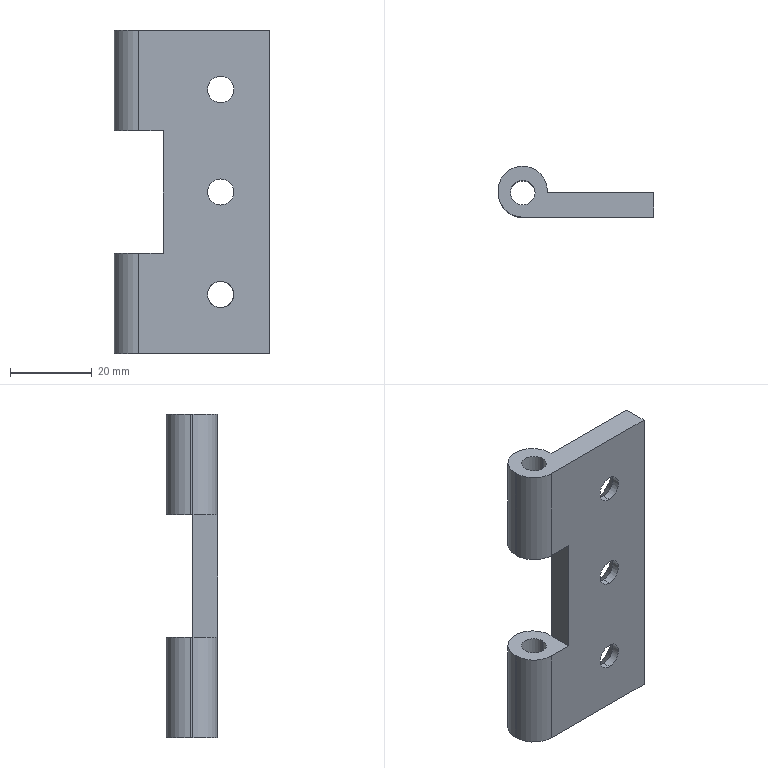Part | SolidWorks | features BaseBody 1 | 1 solid | 32 faces | box 38 x 12.5 x 79 mm | volume 15890 mm3 | cylinder 14 | plane 12 | cone 6 | commonest cylinder face diameters 6.4 x6 6 x4 12 x4
STEP:
#1=CARTESIAN_POINT('',(-20.,1556.,1039.));
#2=VERTEX_POINT('',#1);
#3=CARTESIAN_POINT('',(-26.,1556.,1039.));
#4=VERTEX_POINT('',#3);
#5=CARTESIAN_POINT('',(-23.,1556.,1039.));
#6=DIRECTION('',(0.,0.,-1.));
#7=DIRECTION('',(1.,0.,0.));
#8=AXIS2_PLACEMENT_3D('',#5,#6,#7);
#9=CIRCLE('',#8,3.);
#10=EDGE_CURVE('',#2,#4,#9,.T.);
#11=ORIENTED_EDGE('',*,*,#10,.T.);
#12=CARTESIAN_POINT('',(-26.,1556.,1063.5));
#13=VERTEX_POINT('',#12);
#14=CARTESIAN_POINT('',(-26.,1556.,1039.));
#15=DIRECTION('',(0.,0.,1.));
#16=VECTOR('',#15,1000.);
#17=LINE('',#14,#16);
#18=EDGE_CURVE('',#4,#13,#17,.T.);
#19=ORIENTED_EDGE('',*,*,#18,.T.);
#20=CARTESIAN_POINT('',(-20.,1556.,1063.5));
#21=VERTEX_POINT('',#20);
#22=CARTESIAN_POINT('',(-23.,1556.,1063.5));
#23=DIRECTION('',(0.,0.,1.));
#24=DIRECTION('',(1.,0.,0.));
#25=AXIS2_PLACEMENT_3D('',#22,#23,#24);
#26=CIRCLE('',#25,3.);
#27=EDGE_CURVE('',#13,#21,#26,.T.);
#28=ORIENTED_EDGE('',*,*,#27,.T.);
#29=CARTESIAN_POINT('',(-20.,1556.,1039.));
#30=DIRECTION('',(0.,0.,1.));
#31=VECTOR('',#30,1000.);
#32=LINE('',#29,#31);
#33=EDGE_CURVE('',#2,#21,#32,.T.);
#34=ORIENTED_EDGE('',*,*,#33,.F.);
#35=EDGE_LOOP('',(#11,#19,#28,#34));
#36=FACE_OUTER_BOUND('',#35,.T.);
#37=CARTESIAN_POINT('',(-23.,1556.,1039.));
#38=DIRECTION('',(0.,0.,1.));
#39=DIRECTION('',(1.,0.,0.));
#40=AXIS2_PLACEMENT_3D('',#37,#38,#39);
#41=CYLINDRICAL_SURFACE('',#40,3.);
#42=ADVANCED_FACE('',(#36),#41,.F.);
#43=CARTESIAN_POINT('',(-3.,1552.,1081.7));
#44=VERTEX_POINT('',#43);
#45=CARTESIAN_POINT('',(-3.,1552.,1075.3));
#46=VERTEX_POINT('',#45);
#47=CARTESIAN_POINT('',(-3.,1552.,1078.5));
#48=DIRECTION('',(0.,-1.,0.));
#49=DIRECTION('',(0.,0.,-1.));
#50=AXIS2_PLACEMENT_3D('',#47,#48,#49);
#51=CIRCLE('',#50,3.2);
#52=EDGE_CURVE('',#44,#46,#51,.T.);
#53=ORIENTED_EDGE('',*,*,#52,.T.);
#54=CARTESIAN_POINT('',(-3.,1556.,1071.3));
#55=VERTEX_POINT('',#54);
#56=CARTESIAN_POINT('',(-3.,1552.,1075.3));
#57=DIRECTION('',(0.,0.7071,-0.7071));
#58=VECTOR('',#57,1000.);
#59=LINE('',#56,#58);
#60=EDGE_CURVE('',#46,#55,#59,.T.);
#61=ORIENTED_EDGE('',*,*,#60,.T.);
#62=CARTESIAN_POINT('',(-3.,1556.,1085.7));
#63=VERTEX_POINT('',#62);
#64=CARTESIAN_POINT('',(-3.,1556.,1078.5));
#65=DIRECTION('',(0.,-1.,0.));
#66=DIRECTION('',(0.,0.,1.));
#67=AXIS2_PLACEMENT_3D('',#64,#65,#66);
#68=CIRCLE('',#67,7.2);
#69=EDGE_CURVE('',#63,#55,#68,.T.);
#70=ORIENTED_EDGE('',*,*,#69,.F.);
#71=CARTESIAN_POINT('',(-3.,1552.,1081.7));
#72=DIRECTION('',(0.,0.7071,0.7071));
#73=VECTOR('',#72,1000.);
#74=LINE('',#71,#73);
#75=EDGE_CURVE('',#44,#63,#74,.T.);
#76=ORIENTED_EDGE('',*,*,#75,.F.);
#77=EDGE_LOOP('',(#53,#61,#70,#76));
#78=FACE_OUTER_BOUND('',#77,.T.);
#79=CARTESIAN_POINT('',(-3.,1552.,1078.5));
#80=DIRECTION('',(0.,1.,0.));
#81=DIRECTION('',(0.,0.,1.));
#82=AXIS2_PLACEMENT_3D('',#79,#80,#81);
#83=CONICAL_SURFACE('',#82,3.2,0.7854);
#84=ADVANCED_FACE('',(#78),#83,.F.);
#85=CARTESIAN_POINT('',(-3.,1552.,1106.7));
#86=VERTEX_POINT('',#85);
#87=CARTESIAN_POINT('',(-3.,1552.,1100.3));
#88=VERTEX_POINT('',#87);
#89=CARTESIAN_POINT('',(-3.,1552.,1103.5));
#90=DIRECTION('',(0.,-1.,0.));
#91=DIRECTION('',(0.,0.,-1.));
#92=AXIS2_PLACEMENT_3D('',#89,#90,#91);
#93=CIRCLE('',#92,3.2);
#94=EDGE_CURVE('',#86,#88,#93,.T.);
#95=ORIENTED_EDGE('',*,*,#94,.T.);
#96=CARTESIAN_POINT('',(-3.,1556.,1096.3));
#97=VERTEX_POINT('',#96);
#98=CARTESIAN_POINT('',(-3.,1552.,1100.3));
#99=DIRECTION('',(0.,0.7071,-0.7071));
#100=VECTOR('',#99,1000.);
#101=LINE('',#98,#100);
#102=EDGE_CURVE('',#88,#97,#101,.T.);
#103=ORIENTED_EDGE('',*,*,#102,.T.);
#104=CARTESIAN_POINT('',(-3.,1556.,1110.7));
#105=VERTEX_POINT('',#104);
#106=CARTESIAN_POINT('',(-3.,1556.,1103.5));
#107=DIRECTION('',(0.,-1.,0.));
#108=DIRECTION('',(0.,0.,1.));
#109=AXIS2_PLACEMENT_3D('',#106,#107,#108);
#110=CIRCLE('',#109,7.2);
#111=EDGE_CURVE('',#105,#97,#110,.T.);
#112=ORIENTED_EDGE('',*,*,#111,.F.);
#113=CARTESIAN_POINT('',(-3.,1552.,1106.7));
#114=DIRECTION('',(0.,0.7071,0.7071));
#115=VECTOR('',#114,1000.);
#116=LINE('',#113,#115);
#117=EDGE_CURVE('',#86,#105,#116,.T.);
#118=ORIENTED_EDGE('',*,*,#117,.F.);
#119=EDGE_LOOP('',(#95,#103,#112,#118));
#120=FACE_OUTER_BOUND('',#119,.T.);
#121=CARTESIAN_POINT('',(-3.,1552.,1103.5));
#122=DIRECTION('',(0.,1.,0.));
#123=DIRECTION('',(0.,0.,1.));
#124=AXIS2_PLACEMENT_3D('',#121,#122,#123);
#125=CONICAL_SURFACE('',#124,3.2,0.7854);
#126=ADVANCED_FACE('',(#120),#125,.F.);
#127=CARTESIAN_POINT('',(-3.,1552.,1050.3));
#128=VERTEX_POINT('',#127);
#129=CARTESIAN_POINT('',(0.2,1552.,1053.5));
#130=VERTEX_POINT('',#129);
#131=CARTESIAN_POINT('',(-3.,1552.,1053.5));
#132=DIRECTION('',(0.,-1.,0.));
#133=DIRECTION('',(0.,0.,-1.));
#134=AXIS2_PLACEMENT_3D('',#131,#132,#133);
#135=CIRCLE('',#134,3.2);
#136=EDGE_CURVE('',#128,#130,#135,.T.);
#137=ORIENTED_EDGE('',*,*,#136,.T.);
#138=CARTESIAN_POINT('',(4.2,1556.,1053.5));
#139=VERTEX_POINT('',#138);
#140=CARTESIAN_POINT('',(0.2,1552.,1053.5));
#141=DIRECTION('',(0.7071,0.7071,0.));
#142=VECTOR('',#141,1000.);
#143=LINE('',#140,#142);
#144=EDGE_CURVE('',#130,#139,#143,.T.);
#145=ORIENTED_EDGE('',*,*,#144,.T.);
#146=CARTESIAN_POINT('',(-10.2,1556.,1053.5));
#147=VERTEX_POINT('',#146);
#148=CARTESIAN_POINT('',(-3.,1556.,1053.5));
#149=DIRECTION('',(0.,-1.,0.));
#150=DIRECTION('',(-1.,0.,0.));
#151=AXIS2_PLACEMENT_3D('',#148,#149,#150);
#152=CIRCLE('',#151,7.2);
#153=EDGE_CURVE('',#147,#139,#152,.T.);
#154=ORIENTED_EDGE('',*,*,#153,.F.);
#155=CARTESIAN_POINT('',(-6.2,1552.,1053.5));
#156=VERTEX_POINT('',#155);
#157=CARTESIAN_POINT('',(-6.2,1552.,1053.5));
#158=DIRECTION('',(-0.7071,0.7071,0.));
#159=VECTOR('',#158,1000.);
#160=LINE('',#157,#159);
#161=EDGE_CURVE('',#156,#147,#160,.T.);
#162=ORIENTED_EDGE('',*,*,#161,.F.);
#163=CARTESIAN_POINT('',(-3.,1552.,1053.5));
#164=DIRECTION('',(0.,-1.,0.));
#165=DIRECTION('',(0.,0.,-1.));
#166=AXIS2_PLACEMENT_3D('',#163,#164,#165);
#167=CIRCLE('',#166,3.2);
#168=EDGE_CURVE('',#156,#128,#167,.T.);
#169=ORIENTED_EDGE('',*,*,#168,.T.);
#170=EDGE_LOOP('',(#137,#145,#154,#162,#169));
#171=FACE_OUTER_BOUND('',#170,.T.);
#172=CARTESIAN_POINT('',(-3.,1552.,1053.5));
#173=DIRECTION('',(0.,1.,0.));
#174=DIRECTION('',(-1.,0.,0.));
#175=AXIS2_PLACEMENT_3D('',#172,#173,#174);
#176=CONICAL_SURFACE('',#175,3.2,0.7854);
#177=ADVANCED_FACE('',(#171),#176,.F.);
#178=CARTESIAN_POINT('',(-3.,1550.,1100.3));
#179=VERTEX_POINT('',#178);
#180=CARTESIAN_POINT('',(-3.,1550.,1106.7));
#181=VERTEX_POINT('',#180);
#182=CARTESIAN_POINT('',(-3.,1550.,1103.5));
#183=DIRECTION('',(0.,1.,0.));
#184=DIRECTION('',(0.,0.,1.));
#185=AXIS2_PLACEMENT_3D('',#182,#183,#184);
#186=CIRCLE('',#185,3.2);
#187=EDGE_CURVE('',#179,#181,#186,.T.);
#188=ORIENTED_EDGE('',*,*,#187,.F.);
#189=CARTESIAN_POINT('',(-3.,1550.,1100.3));
#190=DIRECTION('',(0.,1.,0.));
#191=VECTOR('',#190,1000.);
#192=LINE('',#189,#191);
#193=EDGE_CURVE('',#179,#88,#192,.T.);
#194=ORIENTED_EDGE('',*,*,#193,.T.);
#195=ORIENTED_EDGE('',*,*,#94,.F.);
#196=CARTESIAN_POINT('',(-3.,1550.,1106.7));
#197=DIRECTION('',(0.,1.,0.));
#198=VECTOR('',#197,1000.);
#199=LINE('',#196,#198);
#200=EDGE_CURVE('',#181,#86,#199,.T.);
#201=ORIENTED_EDGE('',*,*,#200,.F.);
#202=EDGE_LOOP('',(#188,#194,#195,#201));
#203=FACE_OUTER_BOUND('',#202,.T.);
#204=CARTESIAN_POINT('',(-3.,1550.,1103.5));
#205=DIRECTION('',(0.,1.,0.));
#206=DIRECTION('',(0.,0.,1.));
#207=AXIS2_PLACEMENT_3D('',#204,#205,#206);
#208=CYLINDRICAL_SURFACE('',#207,3.2);
#209=ADVANCED_FACE('',(#203),#208,.F.);
#210=CARTESIAN_POINT('',(-3.,1550.,1075.3));
#211=VERTEX_POINT('',#210);
#212=CARTESIAN_POINT('',(-3.,1550.,1081.7));
#213=VERTEX_POINT('',#212);
#214=CARTESIAN_POINT('',(-3.,1550.,1078.5));
#215=DIRECTION('',(0.,1.,0.));
#216=DIRECTION('',(0.,0.,1.));
#217=AXIS2_PLACEMENT_3D('',#214,#215,#216);
#218=CIRCLE('',#217,3.2);
#219=EDGE_CURVE('',#211,#213,#218,.T.);
#220=ORIENTED_EDGE('',*,*,#219,.F.);
#221=CARTESIAN_POINT('',(-3.,1550.,1075.3));
#222=DIRECTION('',(0.,1.,0.));
#223=VECTOR('',#222,1000.);
#224=LINE('',#221,#223);
#225=EDGE_CURVE('',#211,#46,#224,.T.);
#226=ORIENTED_EDGE('',*,*,#225,.T.);
#227=ORIENTED_EDGE('',*,*,#52,.F.);
#228=CARTESIAN_POINT('',(-3.,1550.,1081.7));
#229=DIRECTION('',(0.,1.,0.));
#230=VECTOR('',#229,1000.);
#231=LINE('',#228,#230);
#232=EDGE_CURVE('',#213,#44,#231,.T.);
#233=ORIENTED_EDGE('',*,*,#232,.F.);
#234=EDGE_LOOP('',(#220,#226,#227,#233));
#235=FACE_OUTER_BOUND('',#234,.T.);
#236=CARTESIAN_POINT('',(-3.,1550.,1078.5));
#237=DIRECTION('',(0.,1.,0.));
#238=DIRECTION('',(0.,0.,1.));
#239=AXIS2_PLACEMENT_3D('',#236,#237,#238);
#240=CYLINDRICAL_SURFACE('',#239,3.2);
#241=ADVANCED_FACE('',(#235),#240,.F.);
#242=CARTESIAN_POINT('',(-3.,1550.,1050.3));
#243=VERTEX_POINT('',#242);
#244=CARTESIAN_POINT('',(-3.,1550.,1056.7));
#245=VERTEX_POINT('',#244);
#246=CARTESIAN_POINT('',(-3.,1550.,1053.5));
#247=DIRECTION('',(0.,1.,0.));
#248=DIRECTION('',(0.,0.,1.));
#249=AXIS2_PLACEMENT_3D('',#246,#247,#248);
#250=CIRCLE('',#249,3.2);
#251=EDGE_CURVE('',#243,#245,#250,.T.);
#252=ORIENTED_EDGE('',*,*,#251,.F.);
#253=CARTESIAN_POINT('',(-3.,1550.,1050.3));
#254=DIRECTION('',(0.,1.,0.));
#255=VECTOR('',#254,1000.);
#256=LINE('',#253,#255);
#257=EDGE_CURVE('',#243,#128,#256,.T.);
#258=ORIENTED_EDGE('',*,*,#257,.T.);
#259=ORIENTED_EDGE('',*,*,#168,.F.);
#260=CARTESIAN_POINT('',(-3.,1552.,1056.7));
#261=VERTEX_POINT('',#260);
#262=CARTESIAN_POINT('',(-3.,1552.,1053.5));
#263=DIRECTION('',(0.,-1.,0.));
#264=DIRECTION('',(0.,0.,-1.));
#265=AXIS2_PLACEMENT_3D('',#262,#263,#264);
#266=CIRCLE('',#265,3.2);
#267=EDGE_CURVE('',#261,#156,#266,.T.);
#268=ORIENTED_EDGE('',*,*,#267,.F.);
#269=CARTESIAN_POINT('',(-3.,1550.,1056.7));
#270=DIRECTION('',(0.,1.,0.));
#271=VECTOR('',#270,1000.);
#272=LINE('',#269,#271);
#273=EDGE_CURVE('',#245,#261,#272,.T.);
#274=ORIENTED_EDGE('',*,*,#273,.F.);
#275=EDGE_LOOP('',(#252,#258,#259,#268,#274));
#276=FACE_OUTER_BOUND('',#275,.T.);
#277=CARTESIAN_POINT('',(-3.,1550.,1053.5));
#278=DIRECTION('',(0.,1.,0.));
#279=DIRECTION('',(0.,0.,1.));
#280=AXIS2_PLACEMENT_3D('',#277,#278,#279);
#281=CYLINDRICAL_SURFACE('',#280,3.2);
#282=ADVANCED_FACE('',(#276),#281,.F.);
#283=CARTESIAN_POINT('',(-20.,1556.,1093.5));
#284=VERTEX_POINT('',#283);
#285=CARTESIAN_POINT('',(-26.,1556.,1093.5));
#286=VERTEX_POINT('',#285);
#287=CARTESIAN_POINT('',(-23.,1556.,1093.5));
#288=DIRECTION('',(0.,0.,-1.));
#289=DIRECTION('',(1.,0.,0.));
#290=AXIS2_PLACEMENT_3D('',#287,#288,#289);
#291=CIRCLE('',#290,3.);
#292=EDGE_CURVE('',#284,#286,#291,.T.);
#293=ORIENTED_EDGE('',*,*,#292,.T.);
#294=CARTESIAN_POINT('',(-26.,1556.,1118.));
#295=VERTEX_POINT('',#294);
#296=CARTESIAN_POINT('',(-26.,1556.,1093.5));
#297=DIRECTION('',(0.,0.,1.));
#298=VECTOR('',#297,1000.);
#299=LINE('',#296,#298);
#300=EDGE_CURVE('',#286,#295,#299,.T.);
#301=ORIENTED_EDGE('',*,*,#300,.T.);
#302=CARTESIAN_POINT('',(-20.,1556.,1118.));
#303=VERTEX_POINT('',#302);
#304=CARTESIAN_POINT('',(-23.,1556.,1118.));
#305=DIRECTION('',(0.,0.,-1.));
#306=DIRECTION('',(1.,0.,0.));
#307=AXIS2_PLACEMENT_3D('',#304,#305,#306);
#308=CIRCLE('',#307,3.);
#309=EDGE_CURVE('',#303,#295,#308,.T.);
#310=ORIENTED_EDGE('',*,*,#309,.F.);
#311=CARTESIAN_POINT('',(-20.,1556.,1093.5));
#312=DIRECTION('',(0.,0.,1.));
#313=VECTOR('',#312,1000.);
#314=LINE('',#311,#313);
#315=EDGE_CURVE('',#284,#303,#314,.T.);
#316=ORIENTED_EDGE('',*,*,#315,.F.);
#317=EDGE_LOOP('',(#293,#301,#310,#316));
#318=FACE_OUTER_BOUND('',#317,.T.);
#319=CARTESIAN_POINT('',(-23.,1556.,1093.5));
#320=DIRECTION('',(0.,0.,1.));
#321=DIRECTION('',(1.,0.,0.));
#322=AXIS2_PLACEMENT_3D('',#319,#320,#321);
#323=CYLINDRICAL_SURFACE('',#322,3.);
#324=ADVANCED_FACE('',(#318),#323,.F.);
#325=ORIENTED_EDGE('',*,*,#10,.F.);
#326=CARTESIAN_POINT('',(-23.,1556.,1039.));
#327=DIRECTION('',(0.,0.,-1.));
#328=DIRECTION('',(1.,0.,0.));
#329=AXIS2_PLACEMENT_3D('',#326,#327,#328);
#330=CIRCLE('',#329,3.);
#331=EDGE_CURVE('',#4,#2,#330,.T.);
#332=ORIENTED_EDGE('',*,*,#331,.F.);
#333=EDGE_LOOP('',(#325,#332));
#334=FACE_BOUND('',#333,.T.);
#335=CARTESIAN_POINT('',(-17.,1556.5,1039.));
#336=VERTEX_POINT('',#335);
#337=CARTESIAN_POINT('',(-29.,1556.5,1039.));
#338=VERTEX_POINT('',#337);
#339=CARTESIAN_POINT('',(-23.,1556.5,1039.));
#340=DIRECTION('',(0.,0.,1.));
#341=DIRECTION('',(-1.,0.,0.));
#342=AXIS2_PLACEMENT_3D('',#339,#340,#341);
#343=CIRCLE('',#342,6.);
#344=EDGE_CURVE('',#336,#338,#343,.T.);
#345=ORIENTED_EDGE('',*,*,#344,.F.);
#346=CARTESIAN_POINT('',(-17.,1556.,1039.));
#347=VERTEX_POINT('',#346);
#348=CARTESIAN_POINT('',(-17.,1556.25,1039.));
#349=DIRECTION('',(0.,1.,0.));
#350=VECTOR('',#349,1000.);
#351=LINE('',#348,#350);
#352=EDGE_CURVE('',#347,#336,#351,.T.);
#353=ORIENTED_EDGE('',*,*,#352,.F.);
#354=CARTESIAN_POINT('',(9.,1556.,1039.));
#355=VERTEX_POINT('',#354);
#356=CARTESIAN_POINT('',(-10.,1556.,1039.));
#357=DIRECTION('',(-1.,0.,0.));
#358=VECTOR('',#357,1000.);
#359=LINE('',#356,#358);
#360=EDGE_CURVE('',#355,#347,#359,.T.);
#361=ORIENTED_EDGE('',*,*,#360,.F.);
#362=CARTESIAN_POINT('',(9.,1550.,1039.));
#363=VERTEX_POINT('',#362);
#364=CARTESIAN_POINT('',(9.,1556.25,1039.));
#365=DIRECTION('',(0.,1.,0.));
#366=VECTOR('',#365,1000.);
#367=LINE('',#364,#366);
#368=EDGE_CURVE('',#363,#355,#367,.T.);
#369=ORIENTED_EDGE('',*,*,#368,.F.);
#370=CARTESIAN_POINT('',(-23.,1550.,1039.));
#371=VERTEX_POINT('',#370);
#372=CARTESIAN_POINT('',(-10.,1550.,1039.));
#373=DIRECTION('',(1.,0.,0.));
#374=VECTOR('',#373,1000.);
#375=LINE('',#372,#374);
#376=EDGE_CURVE('',#371,#363,#375,.T.);
#377=ORIENTED_EDGE('',*,*,#376,.F.);
#378=CARTESIAN_POINT('',(-29.,1556.,1039.));
#379=VERTEX_POINT('',#378);
#380=CARTESIAN_POINT('',(-23.,1556.,1039.));
#381=DIRECTION('',(0.,0.,1.));
#382=DIRECTION('',(-1.,0.,0.));
#383=AXIS2_PLACEMENT_3D('',#380,#381,#382);
#384=CIRCLE('',#383,6.);
#385=EDGE_CURVE('',#379,#371,#384,.T.);
#386=ORIENTED_EDGE('',*,*,#385,.F.);
#387=CARTESIAN_POINT('',(-29.,1556.25,1039.));
#388=DIRECTION('',(0.,-1.,0.));
#389=VECTOR('',#388,1000.);
#390=LINE('',#387,#389);
#391=EDGE_CURVE('',#338,#379,#390,.T.);
#392=ORIENTED_EDGE('',*,*,#391,.F.);
#393=EDGE_LOOP('',(#345,#353,#361,#369,#377,#386,#392));
#394=FACE_OUTER_BOUND('',#393,.T.);
#395=CARTESIAN_POINT('',(-29.76,1549.75,1039.));
#396=DIRECTION('',(0.,0.,1.));
#397=DIRECTION('',(1.,0.,0.));
#398=AXIS2_PLACEMENT_3D('',#395,#396,#397);
#399=PLANE('',#398);
#400=ADVANCED_FACE('',(#334,#394),#399,.F.);
#401=ORIENTED_EDGE('',*,*,#18,.F.);
#402=ORIENTED_EDGE('',*,*,#331,.T.);
#403=ORIENTED_EDGE('',*,*,#33,.T.);
#404=CARTESIAN_POINT('',(-23.,1556.,1063.5));
#405=DIRECTION('',(0.,0.,1.));
#406=DIRECTION('',(1.,0.,0.));
#407=AXIS2_PLACEMENT_3D('',#404,#405,#406);
#408=CIRCLE('',#407,3.);
#409=EDGE_CURVE('',#21,#13,#408,.T.);
#410=ORIENTED_EDGE('',*,*,#409,.T.);
#411=EDGE_LOOP('',(#401,#402,#403,#410));
#412=FACE_OUTER_BOUND('',#411,.T.);
#413=CARTESIAN_POINT('',(-23.,1556.,1039.));
#414=DIRECTION('',(0.,0.,1.));
#415=DIRECTION('',(1.,0.,0.));
#416=AXIS2_PLACEMENT_3D('',#413,#414,#415);
#417=CYLINDRICAL_SURFACE('',#416,3.);
#418=ADVANCED_FACE('',(#412),#417,.F.);
#419=CARTESIAN_POINT('',(-17.,1556.5,1063.5));
#420=VERTEX_POINT('',#419);
#421=CARTESIAN_POINT('',(-29.,1556.5,1063.5));
#422=VERTEX_POINT('',#421);
#423=CARTESIAN_POINT('',(-23.,1556.5,1063.5));
#424=DIRECTION('',(0.,0.,1.));
#425=DIRECTION('',(-1.,0.,0.));
#426=AXIS2_PLACEMENT_3D('',#423,#424,#425);
#427=CIRCLE('',#426,6.);
#428=EDGE_CURVE('',#420,#422,#427,.T.);
#429=ORIENTED_EDGE('',*,*,#428,.F.);
#430=CARTESIAN_POINT('',(-17.,1556.5,1051.25));
#431=DIRECTION('',(0.,0.,1.));
#432=VECTOR('',#431,1000.);
#433=LINE('',#430,#432);
#434=EDGE_CURVE('',#336,#420,#433,.T.);
#435=ORIENTED_EDGE('',*,*,#434,.F.);
#436=ORIENTED_EDGE('',*,*,#344,.T.);
#437=CARTESIAN_POINT('',(-29.,1556.5,1051.25));
#438=DIRECTION('',(0.,0.,-1.));
#439=VECTOR('',#438,1000.);
#440=LINE('',#437,#439);
#441=EDGE_CURVE('',#422,#338,#440,.T.);
#442=ORIENTED_EDGE('',*,*,#441,.F.);
#443=EDGE_LOOP('',(#429,#435,#436,#442));
#444=FACE_OUTER_BOUND('',#443,.T.);
#445=CARTESIAN_POINT('',(-23.,1556.5,1063.5));
#446=DIRECTION('',(0.,0.,-1.));
#447=DIRECTION('',(-1.,0.,0.));
#448=AXIS2_PLACEMENT_3D('',#445,#446,#447);
#449=CYLINDRICAL_SURFACE('',#448,6.);
#450=ADVANCED_FACE('',(#444),#449,.T.);
#451=ORIENTED_EDGE('',*,*,#69,.T.);
#452=CARTESIAN_POINT('',(-3.,1556.,1078.5));
#453=DIRECTION('',(0.,-1.,0.));
#454=DIRECTION('',(0.,0.,1.));
#455=AXIS2_PLACEMENT_3D('',#452,#453,#454);
#456=CIRCLE('',#455,7.2);
#457=EDGE_CURVE('',#55,#63,#456,.T.);
#458=ORIENTED_EDGE('',*,*,#457,.T.);
#459=EDGE_LOOP('',(#451,#458));
#460=FACE_BOUND('',#459,.T.);
#461=ORIENTED_EDGE('',*,*,#111,.T.);
#462=CARTESIAN_POINT('',(-3.,1556.,1103.5));
#463=DIRECTION('',(0.,-1.,0.));
#464=DIRECTION('',(0.,0.,1.));
#465=AXIS2_PLACEMENT_3D('',#462,#463,#464);
#466=CIRCLE('',#465,7.2);
#467=EDGE_CURVE('',#97,#105,#466,.T.);
#468=ORIENTED_EDGE('',*,*,#467,.T.);
#469=EDGE_LOOP('',(#461,#468));
#470=FACE_BOUND('',#469,.T.);
#471=ORIENTED_EDGE('',*,*,#153,.T.);
#472=CARTESIAN_POINT('',(-3.,1556.,1053.5));
#473=DIRECTION('',(0.,-1.,0.));
#474=DIRECTION('',(-1.,0.,0.));
#475=AXIS2_PLACEMENT_3D('',#472,#473,#474);
#476=CIRCLE('',#475,7.2);
#477=EDGE_CURVE('',#139,#147,#476,.T.);
#478=ORIENTED_EDGE('',*,*,#477,.T.);
#479=EDGE_LOOP('',(#471,#478));
#480=FACE_BOUND('',#479,.T.);
#481=CARTESIAN_POINT('',(9.,1556.,1118.));
#482=VERTEX_POINT('',#481);
#483=CARTESIAN_POINT('',(9.,1556.,1078.5));
#484=DIRECTION('',(0.,0.,-1.));
#485=VECTOR('',#484,1000.);
#486=LINE('',#483,#485);
#487=EDGE_CURVE('',#482,#355,#486,.T.);
#488=ORIENTED_EDGE('',*,*,#487,.T.);
#489=ORIENTED_EDGE('',*,*,#360,.T.);
#490=CARTESIAN_POINT('',(-17.,1556.,1063.5));
#491=VERTEX_POINT('',#490);
#492=CARTESIAN_POINT('',(-17.,1556.,1078.5));
#493=DIRECTION('',(0.,0.,1.));
#494=VECTOR('',#493,1000.);
#495=LINE('',#492,#494);
#496=EDGE_CURVE('',#347,#491,#495,.T.);
#497=ORIENTED_EDGE('',*,*,#496,.T.);
#498=CARTESIAN_POINT('',(-17.,1556.,1093.5));
#499=VERTEX_POINT('',#498);
#500=CARTESIAN_POINT('',(-17.,1556.,1078.5));
#501=DIRECTION('',(0.,0.,1.));
#502=VECTOR('',#501,1000.);
#503=LINE('',#500,#502);
#504=EDGE_CURVE('',#491,#499,#503,.T.);
#505=ORIENTED_EDGE('',*,*,#504,.T.);
#506=CARTESIAN_POINT('',(-17.,1556.,1118.));
#507=VERTEX_POINT('',#506);
#508=CARTESIAN_POINT('',(-17.,1556.,1078.5));
#509=DIRECTION('',(0.,0.,1.));
#510=VECTOR('',#509,1000.);
#511=LINE('',#508,#510);
#512=EDGE_CURVE('',#499,#507,#511,.T.);
#513=ORIENTED_EDGE('',*,*,#512,.T.);
#514=CARTESIAN_POINT('',(-4.,1556.,1118.));
#515=DIRECTION('',(1.,0.,0.));
#516=VECTOR('',#515,1000.);
#517=LINE('',#514,#516);
#518=EDGE_CURVE('',#507,#482,#517,.T.);
#519=ORIENTED_EDGE('',*,*,#518,.T.);
#520=EDGE_LOOP('',(#488,#489,#497,#505,#513,#519));
#521=FACE_OUTER_BOUND('',#520,.T.);
#522=CARTESIAN_POINT('',(9.52,1556.,1037.42));
#523=DIRECTION('',(0.,1.,0.));
#524=DIRECTION('',(-1.,0.,0.));
#525=AXIS2_PLACEMENT_3D('',#522,#523,#524);
#526=PLANE('',#525);
#527=ADVANCED_FACE('',(#460,#470,#480,#521),#526,.T.);
#528=CARTESIAN_POINT('',(9.,1550.,1118.));
#529=VERTEX_POINT('',#528);
#530=CARTESIAN_POINT('',(9.,1553.,1118.));
#531=DIRECTION('',(0.,-1.,0.));
#532=VECTOR('',#531,1000.);
#533=LINE('',#530,#532);
#534=EDGE_CURVE('',#482,#529,#533,.T.);
#535=ORIENTED_EDGE('',*,*,#534,.T.);
#536=CARTESIAN_POINT('',(9.,1550.,1078.5));
#537=DIRECTION('',(0.,0.,-1.));
#538=VECTOR('',#537,1000.);
#539=LINE('',#536,#538);
#540=EDGE_CURVE('',#529,#363,#539,.T.);
#541=ORIENTED_EDGE('',*,*,#540,.T.);
#542=ORIENTED_EDGE('',*,*,#368,.T.);
#543=ORIENTED_EDGE('',*,*,#487,.F.);
#544=EDGE_LOOP('',(#535,#541,#542,#543));
#545=FACE_OUTER_BOUND('',#544,.T.);
#546=CARTESIAN_POINT('',(9.,1549.88,1037.42));
#547=DIRECTION('',(1.,0.,0.));
#548=DIRECTION('',(0.,1.,0.));
#549=AXIS2_PLACEMENT_3D('',#546,#547,#548);
#550=PLANE('',#549);
#551=ADVANCED_FACE('',(#545),#550,.T.);
#552=CARTESIAN_POINT('',(-3.,1550.,1103.5));
#553=DIRECTION('',(0.,1.,0.));
#554=DIRECTION('',(0.,0.,1.));
#555=AXIS2_PLACEMENT_3D('',#552,#553,#554);
#556=CIRCLE('',#555,3.2);
#557=EDGE_CURVE('',#181,#179,#556,.T.);
#558=ORIENTED_EDGE('',*,*,#557,.T.);
#559=ORIENTED_EDGE('',*,*,#187,.T.);
#560=EDGE_LOOP('',(#558,#559));
#561=FACE_BOUND('',#560,.T.);
#562=CARTESIAN_POINT('',(-3.,1550.,1078.5));
#563=DIRECTION('',(0.,1.,0.));
#564=DIRECTION('',(0.,0.,1.));
#565=AXIS2_PLACEMENT_3D('',#562,#563,#564);
#566=CIRCLE('',#565,3.2);
#567=EDGE_CURVE('',#213,#211,#566,.T.);
#568=ORIENTED_EDGE('',*,*,#567,.T.);
#569=ORIENTED_EDGE('',*,*,#219,.T.);
#570=EDGE_LOOP('',(#568,#569));
#571=FACE_BOUND('',#570,.T.);
#572=CARTESIAN_POINT('',(-3.,1550.,1053.5));
#573=DIRECTION('',(0.,1.,0.));
#574=DIRECTION('',(0.,0.,1.));
#575=AXIS2_PLACEMENT_3D('',#572,#573,#574);
#576=CIRCLE('',#575,3.2);
#577=EDGE_CURVE('',#245,#243,#576,.T.);
#578=ORIENTED_EDGE('',*,*,#577,.T.);
#579=ORIENTED_EDGE('',*,*,#251,.T.);
#580=EDGE_LOOP('',(#578,#579));
#581=FACE_BOUND('',#580,.T.);
#582=ORIENTED_EDGE('',*,*,#540,.F.);
#583=CARTESIAN_POINT('',(-23.,1550.,1118.));
#584=VERTEX_POINT('',#583);
#585=CARTESIAN_POINT('',(-7.,1550.,1118.));
#586=DIRECTION('',(-1.,0.,0.));
#587=VECTOR('',#586,1000.);
#588=LINE('',#585,#587);
#589=EDGE_CURVE('',#529,#584,#588,.T.);
#590=ORIENTED_EDGE('',*,*,#589,.T.);
#591=CARTESIAN_POINT('',(-23.,1550.,1093.5));
#592=VERTEX_POINT('',#591);
#593=CARTESIAN_POINT('',(-23.,1550.,1078.5));
#594=DIRECTION('',(0.,0.,-1.));
#595=VECTOR('',#594,1000.);
#596=LINE('',#593,#595);
#597=EDGE_CURVE('',#584,#592,#596,.T.);
#598=ORIENTED_EDGE('',*,*,#597,.T.);
#599=CARTESIAN_POINT('',(-17.,1550.,1093.5));
#600=VERTEX_POINT('',#599);
#601=CARTESIAN_POINT('',(-7.,1550.,1093.5));
#602=DIRECTION('',(1.,0.,0.));
#603=VECTOR('',#602,1000.);
#604=LINE('',#601,#603);
#605=EDGE_CURVE('',#592,#600,#604,.T.);
#606=ORIENTED_EDGE('',*,*,#605,.T.);
#607=CARTESIAN_POINT('',(-17.,1550.,1063.5));
#608=VERTEX_POINT('',#607);
#609=CARTESIAN_POINT('',(-17.,1550.,1078.5));
#610=DIRECTION('',(0.,0.,-1.));
#611=VECTOR('',#610,1000.);
#612=LINE('',#609,#611);
#613=EDGE_CURVE('',#600,#608,#612,.T.);
#614=ORIENTED_EDGE('',*,*,#613,.T.);
#615=CARTESIAN_POINT('',(-23.,1550.,1063.5));
#616=VERTEX_POINT('',#615);
#617=CARTESIAN_POINT('',(-7.,1550.,1063.5));
#618=DIRECTION('',(-1.,0.,0.));
#619=VECTOR('',#618,1000.);
#620=LINE('',#617,#619);
#621=EDGE_CURVE('',#608,#616,#620,.T.);
#622=ORIENTED_EDGE('',*,*,#621,.T.);
#623=CARTESIAN_POINT('',(-23.,1550.,1078.5));
#624=DIRECTION('',(0.,0.,-1.));
#625=VECTOR('',#624,1000.);
#626=LINE('',#623,#625);
#627=EDGE_CURVE('',#616,#371,#626,.T.);
#628=ORIENTED_EDGE('',*,*,#627,.T.);
#629=ORIENTED_EDGE('',*,*,#376,.T.);
#630=EDGE_LOOP('',(#582,#590,#598,#606,#614,#622,#628,#629));
#631=FACE_OUTER_BOUND('',#630,.T.);
#632=CARTESIAN_POINT('',(-23.64,1550.,1037.42));
#633=DIRECTION('',(0.,-1.,0.));
#634=DIRECTION('',(1.,0.,0.));
#635=AXIS2_PLACEMENT_3D('',#632,#633,#634);
#636=PLANE('',#635);
#637=ADVANCED_FACE('',(#561,#571,#581,#631),#636,.T.);
#638=CARTESIAN_POINT('',(-29.,1556.,1063.5));
#639=VERTEX_POINT('',#638);
#640=CARTESIAN_POINT('',(-23.,1556.,1063.5));
#641=DIRECTION('',(0.,0.,1.));
#642=DIRECTION('',(-1.,0.,0.));
#643=AXIS2_PLACEMENT_3D('',#640,#641,#642);
#644=CIRCLE('',#643,6.);
#645=EDGE_CURVE('',#639,#616,#644,.T.);
#646=ORIENTED_EDGE('',*,*,#645,.F.);
#647=CARTESIAN_POINT('',(-29.,1556.,1051.25));
#648=DIRECTION('',(0.,0.,1.));
#649=VECTOR('',#648,1000.);
#650=LINE('',#647,#649);
#651=EDGE_CURVE('',#379,#639,#650,.T.);
#652=ORIENTED_EDGE('',*,*,#651,.F.);
#653=ORIENTED_EDGE('',*,*,#385,.T.);
#654=ORIENTED_EDGE('',*,*,#627,.F.);
#655=EDGE_LOOP('',(#646,#652,#653,#654));
#656=FACE_OUTER_BOUND('',#655,.T.);
#657=CARTESIAN_POINT('',(-23.,1556.,1063.5));
#658=DIRECTION('',(0.,0.,-1.));
#659=DIRECTION('',(-1.,0.,0.));
#660=AXIS2_PLACEMENT_3D('',#657,#658,#659);
#661=CYLINDRICAL_SURFACE('',#660,6.);
#662=ADVANCED_FACE('',(#656),#661,.T.);
#663=ORIENTED_EDGE('',*,*,#409,.F.);
#664=ORIENTED_EDGE('',*,*,#27,.F.);
#665=EDGE_LOOP('',(#663,#664));
#666=FACE_BOUND('',#665,.T.);
#667=CARTESIAN_POINT('',(-17.,1556.25,1063.5));
#668=DIRECTION('',(0.,-1.,0.));
#669=VECTOR('',#668,1000.);
#670=LINE('',#667,#669);
#671=EDGE_CURVE('',#491,#608,#670,.T.);
#672=ORIENTED_EDGE('',*,*,#671,.F.);
#673=CARTESIAN_POINT('',(-17.,1556.25,1063.5));
#674=DIRECTION('',(0.,-1.,0.));
#675=VECTOR('',#674,1000.);
#676=LINE('',#673,#675);
#677=EDGE_CURVE('',#420,#491,#676,.T.);
#678=ORIENTED_EDGE('',*,*,#677,.F.);
#679=ORIENTED_EDGE('',*,*,#428,.T.);
#680=CARTESIAN_POINT('',(-29.,1556.25,1063.5));
#681=DIRECTION('',(0.,1.,0.));
#682=VECTOR('',#681,1000.);
#683=LINE('',#680,#682);
#684=EDGE_CURVE('',#639,#422,#683,.T.);
#685=ORIENTED_EDGE('',*,*,#684,.F.);
#686=ORIENTED_EDGE('',*,*,#645,.T.);
#687=ORIENTED_EDGE('',*,*,#621,.F.);
#688=EDGE_LOOP('',(#672,#678,#679,#685,#686,#687));
#689=FACE_OUTER_BOUND('',#688,.T.);
#690=CARTESIAN_POINT('',(-16.76,1549.75,1063.5));
#691=DIRECTION('',(0.,0.,-1.));
#692=DIRECTION('',(-1.,0.,0.));
#693=AXIS2_PLACEMENT_3D('',#690,#691,#692);
#694=PLANE('',#693);
#695=ADVANCED_FACE('',(#666,#689),#694,.F.);
#696=ORIENTED_EDGE('',*,*,#441,.T.);
#697=ORIENTED_EDGE('',*,*,#391,.T.);
#698=ORIENTED_EDGE('',*,*,#651,.T.);
#699=ORIENTED_EDGE('',*,*,#684,.T.);
#700=EDGE_LOOP('',(#696,#697,#698,#699));
#701=FACE_OUTER_BOUND('',#700,.T.);
#702=CARTESIAN_POINT('',(-29.,1556.606,1037.42));
#703=DIRECTION('',(-1.,0.,0.));
#704=DIRECTION('',(0.,-1.,0.));
#705=AXIS2_PLACEMENT_3D('',#702,#703,#704);
#706=PLANE('',#705);
#707=ADVANCED_FACE('',(#701),#706,.T.);
#708=ORIENTED_EDGE('',*,*,#496,.F.);
#709=ORIENTED_EDGE('',*,*,#352,.T.);
#710=ORIENTED_EDGE('',*,*,#434,.T.);
#711=ORIENTED_EDGE('',*,*,#677,.T.);
#712=EDGE_LOOP('',(#708,#709,#710,#711));
#713=FACE_OUTER_BOUND('',#712,.T.);
#714=CARTESIAN_POINT('',(-17.,1555.894,1037.42));
#715=DIRECTION('',(1.,0.,0.));
#716=DIRECTION('',(0.,1.,0.));
#717=AXIS2_PLACEMENT_3D('',#714,#715,#716);
#718=PLANE('',#717);
#719=ADVANCED_FACE('',(#713),#718,.T.);
#720=ORIENTED_EDGE('',*,*,#60,.F.);
#721=CARTESIAN_POINT('',(-3.,1552.,1078.5));
#722=DIRECTION('',(0.,-1.,0.));
#723=DIRECTION('',(0.,0.,-1.));
#724=AXIS2_PLACEMENT_3D('',#721,#722,#723);
#725=CIRCLE('',#724,3.2);
#726=EDGE_CURVE('',#46,#44,#725,.T.);
#727=ORIENTED_EDGE('',*,*,#726,.T.);
#728=ORIENTED_EDGE('',*,*,#75,.T.);
#729=ORIENTED_EDGE('',*,*,#457,.F.);
#730=EDGE_LOOP('',(#720,#727,#728,#729));
#731=FACE_OUTER_BOUND('',#730,.T.);
#732=CARTESIAN_POINT('',(-3.,1552.,1078.5));
#733=DIRECTION('',(0.,1.,0.));
#734=DIRECTION('',(0.,0.,1.));
#735=AXIS2_PLACEMENT_3D('',#732,#733,#734);
#736=CONICAL_SURFACE('',#735,3.2,0.7854);
#737=ADVANCED_FACE('',(#731),#736,.F.);
#738=ORIENTED_EDGE('',*,*,#102,.F.);
#739=CARTESIAN_POINT('',(-3.,1552.,1103.5));
#740=DIRECTION('',(0.,-1.,0.));
#741=DIRECTION('',(0.,0.,-1.));
#742=AXIS2_PLACEMENT_3D('',#739,#740,#741);
#743=CIRCLE('',#742,3.2);
#744=EDGE_CURVE('',#88,#86,#743,.T.);
#745=ORIENTED_EDGE('',*,*,#744,.T.);
#746=ORIENTED_EDGE('',*,*,#117,.T.);
#747=ORIENTED_EDGE('',*,*,#467,.F.);
#748=EDGE_LOOP('',(#738,#745,#746,#747));
#749=FACE_OUTER_BOUND('',#748,.T.);
#750=CARTESIAN_POINT('',(-3.,1552.,1103.5));
#751=DIRECTION('',(0.,1.,0.));
#752=DIRECTION('',(0.,0.,1.));
#753=AXIS2_PLACEMENT_3D('',#750,#751,#752);
#754=CONICAL_SURFACE('',#753,3.2,0.7854);
#755=ADVANCED_FACE('',(#749),#754,.F.);
#756=ORIENTED_EDGE('',*,*,#144,.F.);
#757=CARTESIAN_POINT('',(-3.,1552.,1053.5));
#758=DIRECTION('',(0.,-1.,0.));
#759=DIRECTION('',(0.,0.,-1.));
#760=AXIS2_PLACEMENT_3D('',#757,#758,#759);
#761=CIRCLE('',#760,3.2);
#762=EDGE_CURVE('',#130,#261,#761,.T.);
#763=ORIENTED_EDGE('',*,*,#762,.T.);
#764=ORIENTED_EDGE('',*,*,#267,.T.);
#765=ORIENTED_EDGE('',*,*,#161,.T.);
#766=ORIENTED_EDGE('',*,*,#477,.F.);
#767=EDGE_LOOP('',(#756,#763,#764,#765,#766));
#768=FACE_OUTER_BOUND('',#767,.T.);
#769=CARTESIAN_POINT('',(-3.,1552.,1053.5));
#770=DIRECTION('',(0.,1.,0.));
#771=DIRECTION('',(-1.,0.,0.));
#772=AXIS2_PLACEMENT_3D('',#769,#770,#771);
#773=CONICAL_SURFACE('',#772,3.2,0.7854);
#774=ADVANCED_FACE('',(#768),#773,.F.);
#775=ORIENTED_EDGE('',*,*,#309,.T.);
#776=CARTESIAN_POINT('',(-23.,1556.,1118.));
#777=DIRECTION('',(0.,0.,-1.));
#778=DIRECTION('',(1.,0.,0.));
#779=AXIS2_PLACEMENT_3D('',#776,#777,#778);
#780=CIRCLE('',#779,3.);
#781=EDGE_CURVE('',#295,#303,#780,.T.);
#782=ORIENTED_EDGE('',*,*,#781,.T.);
#783=EDGE_LOOP('',(#775,#782));
#784=FACE_BOUND('',#783,.T.);
#785=CARTESIAN_POINT('',(-17.,1556.5,1118.));
#786=VERTEX_POINT('',#785);
#787=CARTESIAN_POINT('',(-29.,1556.5,1118.));
#788=VERTEX_POINT('',#787);
#789=CARTESIAN_POINT('',(-23.,1556.5,1118.));
#790=DIRECTION('',(0.,0.,1.));
#791=DIRECTION('',(-1.,0.,0.));
#792=AXIS2_PLACEMENT_3D('',#789,#790,#791);
#793=CIRCLE('',#792,6.);
#794=EDGE_CURVE('',#786,#788,#793,.T.);
#795=ORIENTED_EDGE('',*,*,#794,.T.);
#796=CARTESIAN_POINT('',(-29.,1556.,1118.));
#797=VERTEX_POINT('',#796);
#798=CARTESIAN_POINT('',(-29.,1556.25,1118.));
#799=DIRECTION('',(0.,1.,0.));
#800=VECTOR('',#799,1000.);
#801=LINE('',#798,#800);
#802=EDGE_CURVE('',#797,#788,#801,.T.);
#803=ORIENTED_EDGE('',*,*,#802,.F.);
#804=CARTESIAN_POINT('',(-23.,1556.,1118.));
#805=DIRECTION('',(0.,0.,1.));
#806=DIRECTION('',(-1.,0.,0.));
#807=AXIS2_PLACEMENT_3D('',#804,#805,#806);
#808=CIRCLE('',#807,6.);
#809=EDGE_CURVE('',#797,#584,#808,.T.);
#810=ORIENTED_EDGE('',*,*,#809,.T.);
#811=ORIENTED_EDGE('',*,*,#589,.F.);
#812=ORIENTED_EDGE('',*,*,#534,.F.);
#813=ORIENTED_EDGE('',*,*,#518,.F.);
#814=CARTESIAN_POINT('',(-17.,1556.25,1118.));
#815=DIRECTION('',(0.,1.,0.));
#816=VECTOR('',#815,1000.);
#817=LINE('',#814,#816);
#818=EDGE_CURVE('',#507,#786,#817,.T.);
#819=ORIENTED_EDGE('',*,*,#818,.T.);
#820=EDGE_LOOP('',(#795,#803,#810,#811,#812,#813,#819));
#821=FACE_OUTER_BOUND('',#820,.T.);
#822=CARTESIAN_POINT('',(-29.76,1549.75,1118.));
#823=DIRECTION('',(0.,0.,1.));
#824=DIRECTION('',(1.,0.,0.));
#825=AXIS2_PLACEMENT_3D('',#822,#823,#824);
#826=PLANE('',#825);
#827=ADVANCED_FACE('',(#784,#821),#826,.T.);
#828=ORIENTED_EDGE('',*,*,#512,.F.);
#829=CARTESIAN_POINT('',(-17.,1556.5,1093.5));
#830=VERTEX_POINT('',#829);
#831=CARTESIAN_POINT('',(-17.,1556.25,1093.5));
#832=DIRECTION('',(0.,1.,0.));
#833=VECTOR('',#832,1000.);
#834=LINE('',#831,#833);
#835=EDGE_CURVE('',#499,#830,#834,.T.);
#836=ORIENTED_EDGE('',*,*,#835,.T.);
#837=CARTESIAN_POINT('',(-17.,1556.5,1078.5));
#838=DIRECTION('',(0.,0.,1.));
#839=VECTOR('',#838,1000.);
#840=LINE('',#837,#839);
#841=EDGE_CURVE('',#830,#786,#840,.T.);
#842=ORIENTED_EDGE('',*,*,#841,.T.);
#843=ORIENTED_EDGE('',*,*,#818,.F.);
#844=EDGE_LOOP('',(#828,#836,#842,#843));
#845=FACE_OUTER_BOUND('',#844,.T.);
#846=CARTESIAN_POINT('',(-17.,1555.894,1037.42));
#847=DIRECTION('',(1.,0.,0.));
#848=DIRECTION('',(0.,1.,0.));
#849=AXIS2_PLACEMENT_3D('',#846,#847,#848);
#850=PLANE('',#849);
#851=ADVANCED_FACE('',(#845),#850,.T.);
#852=ORIENTED_EDGE('',*,*,#613,.F.);
#853=CARTESIAN_POINT('',(-17.,1553.,1093.5));
#854=DIRECTION('',(0.,-1.,0.));
#855=VECTOR('',#854,1000.);
#856=LINE('',#853,#855);
#857=EDGE_CURVE('',#499,#600,#856,.T.);
#858=ORIENTED_EDGE('',*,*,#857,.F.);
#859=ORIENTED_EDGE('',*,*,#504,.F.);
#860=ORIENTED_EDGE('',*,*,#671,.T.);
#861=EDGE_LOOP('',(#852,#858,#859,#860));
#862=FACE_OUTER_BOUND('',#861,.T.);
#863=CARTESIAN_POINT('',(-17.,1549.88,1094.1));
#864=DIRECTION('',(1.,0.,0.));
#865=DIRECTION('',(0.,0.,-1.));
#866=AXIS2_PLACEMENT_3D('',#863,#864,#865);
#867=PLANE('',#866);
#868=ADVANCED_FACE('',(#862),#867,.F.);
#869=ORIENTED_EDGE('',*,*,#193,.F.);
#870=ORIENTED_EDGE('',*,*,#557,.F.);
#871=ORIENTED_EDGE('',*,*,#200,.T.);
#872=ORIENTED_EDGE('',*,*,#744,.F.);
#873=EDGE_LOOP('',(#869,#870,#871,#872));
#874=FACE_OUTER_BOUND('',#873,.T.);
#875=CARTESIAN_POINT('',(-3.,1550.,1103.5));
#876=DIRECTION('',(0.,1.,0.));
#877=DIRECTION('',(0.,0.,1.));
#878=AXIS2_PLACEMENT_3D('',#875,#876,#877);
#879=CYLINDRICAL_SURFACE('',#878,3.2);
#880=ADVANCED_FACE('',(#874),#879,.F.);
#881=ORIENTED_EDGE('',*,*,#225,.F.);
#882=ORIENTED_EDGE('',*,*,#567,.F.);
#883=ORIENTED_EDGE('',*,*,#232,.T.);
#884=ORIENTED_EDGE('',*,*,#726,.F.);
#885=EDGE_LOOP('',(#881,#882,#883,#884));
#886=FACE_OUTER_BOUND('',#885,.T.);
#887=CARTESIAN_POINT('',(-3.,1550.,1078.5));
#888=DIRECTION('',(0.,1.,0.));
#889=DIRECTION('',(0.,0.,1.));
#890=AXIS2_PLACEMENT_3D('',#887,#888,#889);
#891=CYLINDRICAL_SURFACE('',#890,3.2);
#892=ADVANCED_FACE('',(#886),#891,.F.);
#893=ORIENTED_EDGE('',*,*,#257,.F.);
#894=ORIENTED_EDGE('',*,*,#577,.F.);
#895=ORIENTED_EDGE('',*,*,#273,.T.);
#896=ORIENTED_EDGE('',*,*,#762,.F.);
#897=ORIENTED_EDGE('',*,*,#136,.F.);
#898=EDGE_LOOP('',(#893,#894,#895,#896,#897));
#899=FACE_OUTER_BOUND('',#898,.T.);
#900=CARTESIAN_POINT('',(-3.,1550.,1053.5));
#901=DIRECTION('',(0.,1.,0.));
#902=DIRECTION('',(0.,0.,1.));
#903=AXIS2_PLACEMENT_3D('',#900,#901,#902);
#904=CYLINDRICAL_SURFACE('',#903,3.2);
#905=ADVANCED_FACE('',(#899),#904,.F.);
#906=ORIENTED_EDGE('',*,*,#292,.F.);
#907=CARTESIAN_POINT('',(-23.,1556.,1093.5));
#908=DIRECTION('',(0.,0.,-1.));
#909=DIRECTION('',(1.,0.,0.));
#910=AXIS2_PLACEMENT_3D('',#907,#908,#909);
#911=CIRCLE('',#910,3.);
#912=EDGE_CURVE('',#286,#284,#911,.T.);
#913=ORIENTED_EDGE('',*,*,#912,.F.);
#914=EDGE_LOOP('',(#906,#913));
#915=FACE_BOUND('',#914,.T.);
#916=CARTESIAN_POINT('',(-29.,1556.5,1093.5));
#917=VERTEX_POINT('',#916);
#918=CARTESIAN_POINT('',(-23.,1556.5,1093.5));
#919=DIRECTION('',(0.,0.,1.));
#920=DIRECTION('',(-1.,0.,0.));
#921=AXIS2_PLACEMENT_3D('',#918,#919,#920);
#922=CIRCLE('',#921,6.);
#923=EDGE_CURVE('',#830,#917,#922,.T.);
#924=ORIENTED_EDGE('',*,*,#923,.F.);
#925=ORIENTED_EDGE('',*,*,#835,.F.);
#926=ORIENTED_EDGE('',*,*,#857,.T.);
#927=ORIENTED_EDGE('',*,*,#605,.F.);
#928=CARTESIAN_POINT('',(-29.,1556.,1093.5));
#929=VERTEX_POINT('',#928);
#930=CARTESIAN_POINT('',(-23.,1556.,1093.5));
#931=DIRECTION('',(0.,0.,1.));
#932=DIRECTION('',(-1.,0.,0.));
#933=AXIS2_PLACEMENT_3D('',#930,#931,#932);
#934=CIRCLE('',#933,6.);
#935=EDGE_CURVE('',#929,#592,#934,.T.);
#936=ORIENTED_EDGE('',*,*,#935,.F.);
#937=CARTESIAN_POINT('',(-29.,1556.25,1093.5));
#938=DIRECTION('',(0.,-1.,0.));
#939=VECTOR('',#938,1000.);
#940=LINE('',#937,#939);
#941=EDGE_CURVE('',#917,#929,#940,.T.);
#942=ORIENTED_EDGE('',*,*,#941,.F.);
#943=EDGE_LOOP('',(#924,#925,#926,#927,#936,#942));
#944=FACE_OUTER_BOUND('',#943,.T.);
#945=CARTESIAN_POINT('',(-29.24,1549.75,1093.5));
#946=DIRECTION('',(0.,0.,1.));
#947=DIRECTION('',(1.,0.,0.));
#948=AXIS2_PLACEMENT_3D('',#945,#946,#947);
#949=PLANE('',#948);
#950=ADVANCED_FACE('',(#915,#944),#949,.F.);
#951=ORIENTED_EDGE('',*,*,#809,.F.);
#952=CARTESIAN_POINT('',(-29.,1556.,1105.75));
#953=DIRECTION('',(0.,0.,1.));
#954=VECTOR('',#953,1000.);
#955=LINE('',#952,#954);
#956=EDGE_CURVE('',#929,#797,#955,.T.);
#957=ORIENTED_EDGE('',*,*,#956,.F.);
#958=ORIENTED_EDGE('',*,*,#935,.T.);
#959=ORIENTED_EDGE('',*,*,#597,.F.);
#960=EDGE_LOOP('',(#951,#957,#958,#959));
#961=FACE_OUTER_BOUND('',#960,.T.);
#962=CARTESIAN_POINT('',(-23.,1556.,1118.));
#963=DIRECTION('',(0.,0.,-1.));
#964=DIRECTION('',(-1.,0.,0.));
#965=AXIS2_PLACEMENT_3D('',#962,#963,#964);
#966=CYLINDRICAL_SURFACE('',#965,6.);
#967=ADVANCED_FACE('',(#961),#966,.T.);
#968=ORIENTED_EDGE('',*,*,#300,.F.);
#969=ORIENTED_EDGE('',*,*,#912,.T.);
#970=ORIENTED_EDGE('',*,*,#315,.T.);
#971=ORIENTED_EDGE('',*,*,#781,.F.);
#972=EDGE_LOOP('',(#968,#969,#970,#971));
#973=FACE_OUTER_BOUND('',#972,.T.);
#974=CARTESIAN_POINT('',(-23.,1556.,1093.5));
#975=DIRECTION('',(0.,0.,1.));
#976=DIRECTION('',(1.,0.,0.));
#977=AXIS2_PLACEMENT_3D('',#974,#975,#976);
#978=CYLINDRICAL_SURFACE('',#977,3.);
#979=ADVANCED_FACE('',(#973),#978,.F.);
#980=ORIENTED_EDGE('',*,*,#794,.F.);
#981=ORIENTED_EDGE('',*,*,#841,.F.);
#982=ORIENTED_EDGE('',*,*,#923,.T.);
#983=CARTESIAN_POINT('',(-29.,1556.5,1105.75));
#984=DIRECTION('',(0.,0.,-1.));
#985=VECTOR('',#984,1000.);
#986=LINE('',#983,#985);
#987=EDGE_CURVE('',#788,#917,#986,.T.);
#988=ORIENTED_EDGE('',*,*,#987,.F.);
#989=EDGE_LOOP('',(#980,#981,#982,#988));
#990=FACE_OUTER_BOUND('',#989,.T.);
#991=CARTESIAN_POINT('',(-23.,1556.5,1118.));
#992=DIRECTION('',(0.,0.,-1.));
#993=DIRECTION('',(-1.,0.,0.));
#994=AXIS2_PLACEMENT_3D('',#991,#992,#993);
#995=CYLINDRICAL_SURFACE('',#994,6.);
#996=ADVANCED_FACE('',(#990),#995,.T.);
#997=ORIENTED_EDGE('',*,*,#987,.T.);
#998=ORIENTED_EDGE('',*,*,#941,.T.);
#999=ORIENTED_EDGE('',*,*,#956,.T.);
#1000=ORIENTED_EDGE('',*,*,#802,.T.);
#1001=EDGE_LOOP('',(#997,#998,#999,#1000));
#1002=FACE_OUTER_BOUND('',#1001,.T.);
#1003=CARTESIAN_POINT('',(-29.,1556.606,1037.42));
#1004=DIRECTION('',(-1.,0.,0.));
#1005=DIRECTION('',(0.,-1.,0.));
#1006=AXIS2_PLACEMENT_3D('',#1003,#1004,#1005);
#1007=PLANE('',#1006);
#1008=ADVANCED_FACE('',(#1002),#1007,.T.);
#1009=CLOSED_SHELL('',(#42,#84,#126,#177,#209,#241,#282,#324,#400,#418,#450,#527,#551,#637,#662,#695,#707,#719,#737,#755,#774,#827,#851,#868,#880,#892,#905,#950,#967,#979,#996,#1008));
#1010=MANIFOLD_SOLID_BREP('',#1009);
#1011=CARTESIAN_POINT('',(0.,0.,0.));
#1012=DIRECTION('',(0.,0.,1.));
#1013=DIRECTION('',(1.,0.,0.));
#1014=AXIS2_PLACEMENT_3D('',#1011,#1012,#1013);
#1015=(LENGTH_UNIT()NAMED_UNIT(*)SI_UNIT(.MILLI.,.METRE.));
#1016=UNCERTAINTY_MEASURE_WITH_UNIT(LENGTH_MEASURE(0.00001),#1015,'','');
#1017=(NAMED_UNIT(*)PLANE_ANGLE_UNIT()SI_UNIT($,.RADIAN.));
#1018=(NAMED_UNIT(*)SI_UNIT($,.STERADIAN.)SOLID_ANGLE_UNIT());
#1019=(GEOMETRIC_REPRESENTATION_CONTEXT(3)GLOBAL_UNCERTAINTY_ASSIGNED_CONTEXT((#1016))GLOBAL_UNIT_ASSIGNED_CONTEXT((#1015,#1017,#1018))REPRESENTATION_CONTEXT('',''));
#1020=ADVANCED_BREP_SHAPE_REPRESENTATION('',(#1010,#1014),#1019);